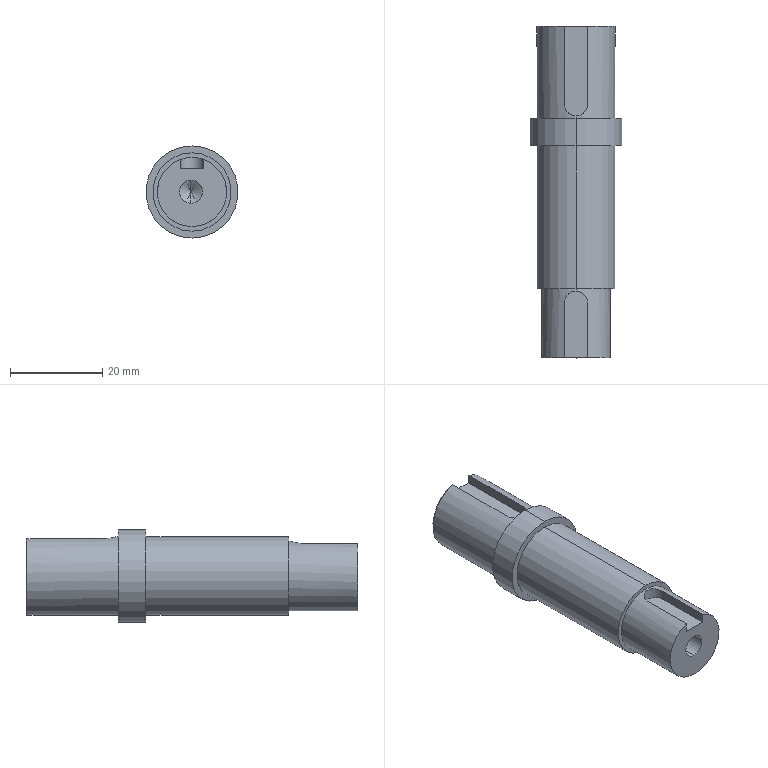Part | STEP file | Cuon T phu H01_2 | 1 solid | 31 faces | box 20 x 72 x 20 mm | volume 15111 mm3 | cylinder 14 | plane 11 | cone 6 | commonest cylinder face diameters 5 x6 17 x4 15 x2 20 x2